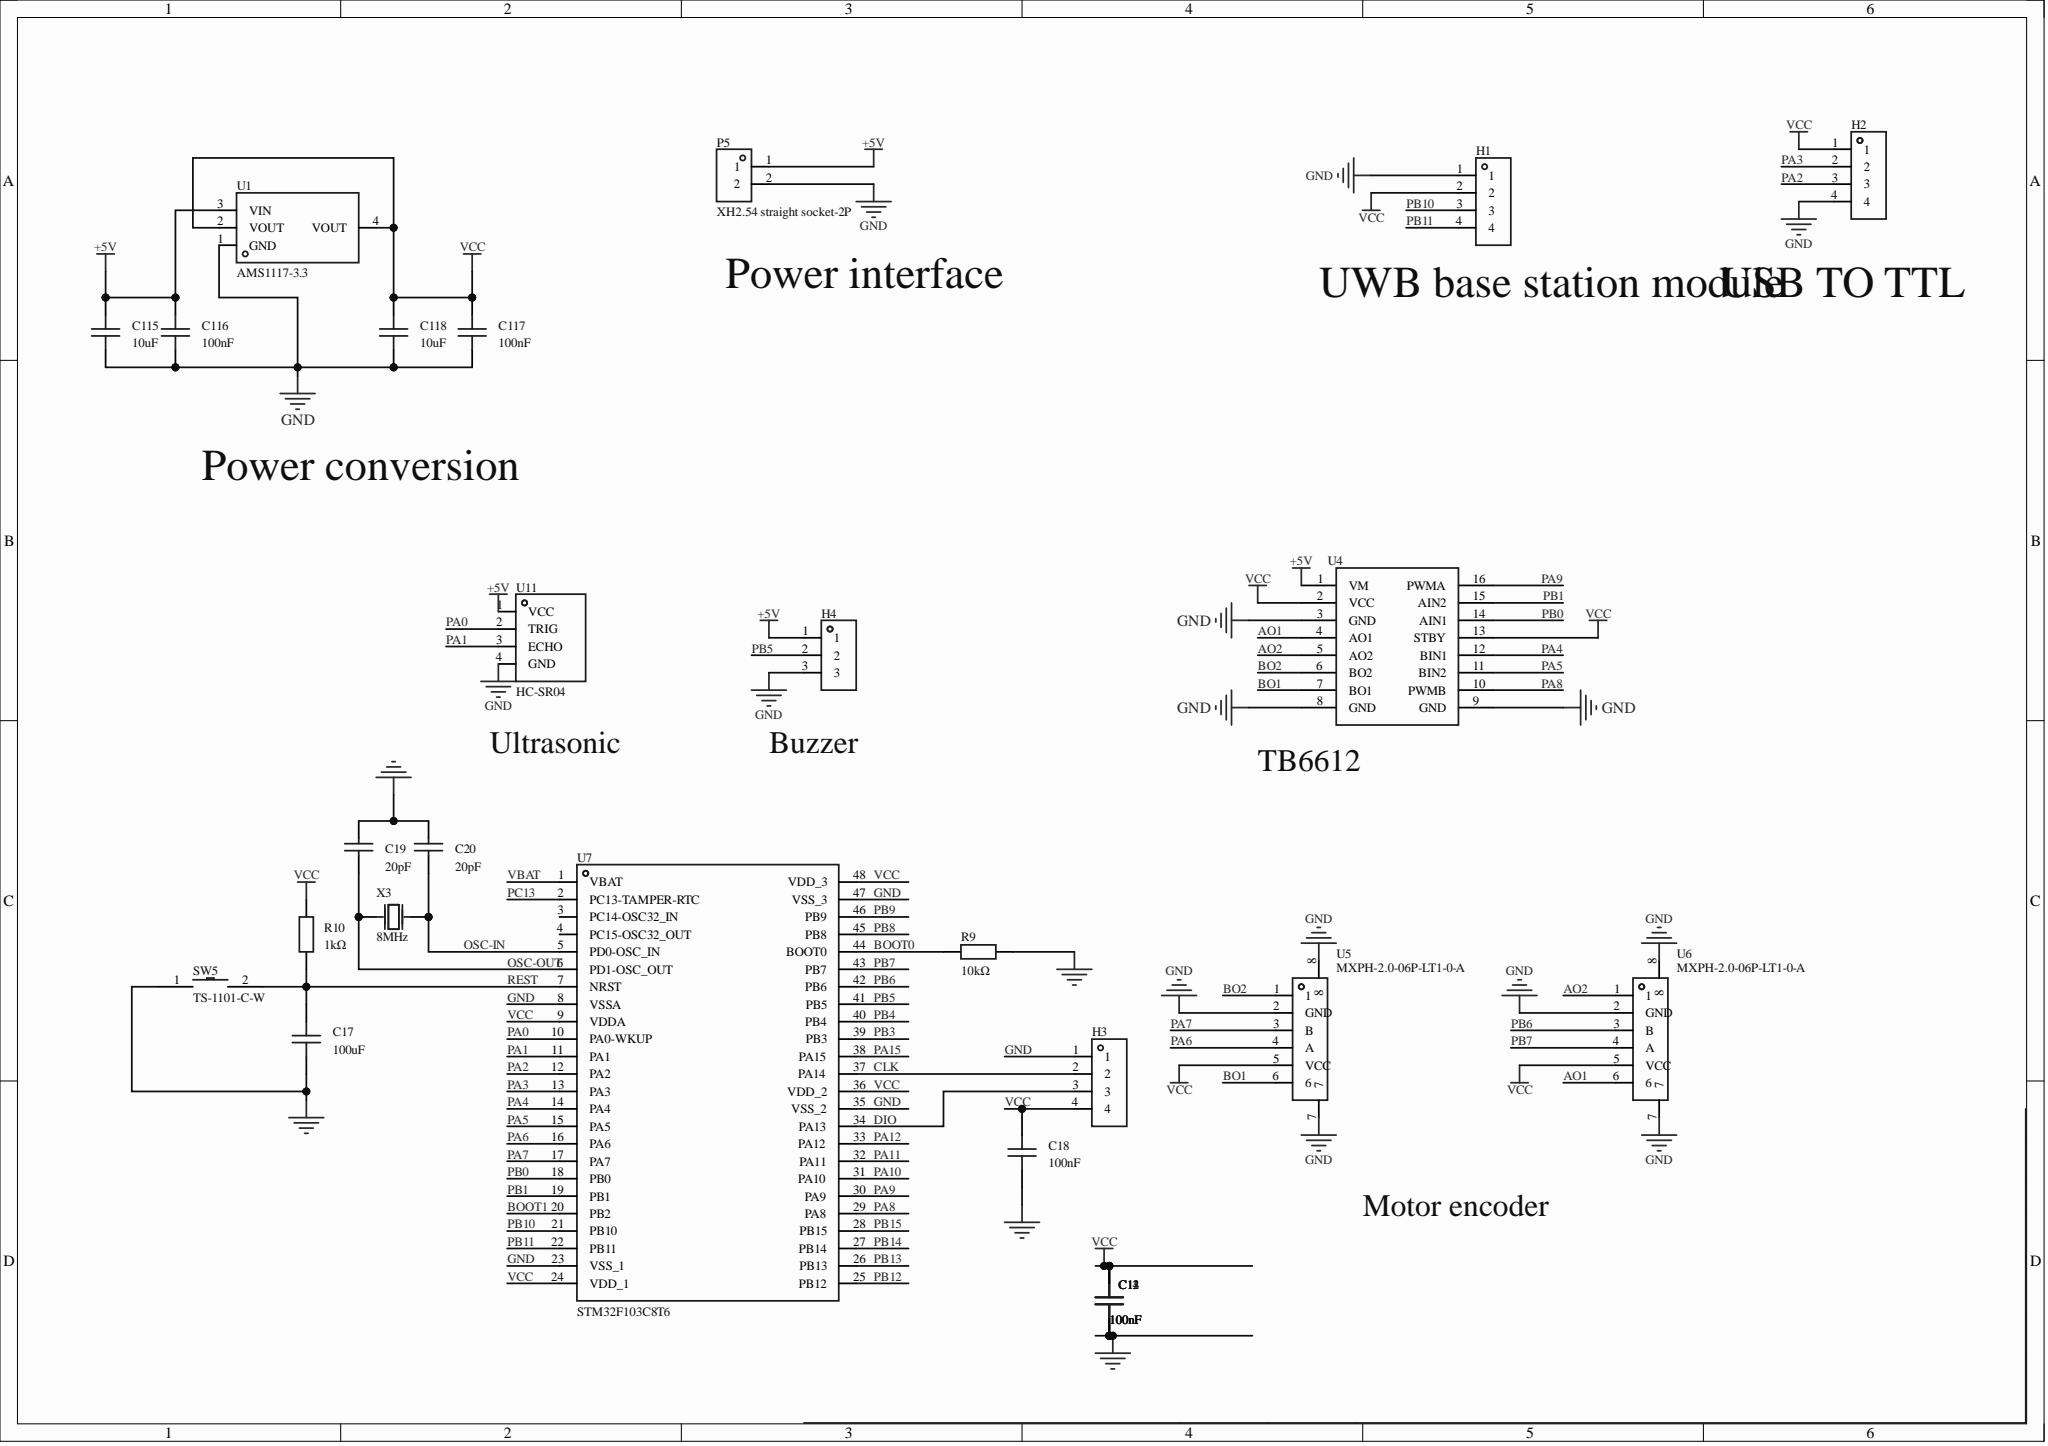Circuit board | Altium Designer | 27 parts | 30 nets
Bill of materials:
Comment,Description,Designator,Footprint,LibRef,Quantity
"100nF","Capacitance: 100nF; tolerance: ±10%; rated voltage: 50V; dielectric (temperature coefficient): X7R;","C11, C12, C13, C14, C18, C116, C117","C0603","CGA0603X7R104K500JT, CC0603KRX7R9BB104","7"
"100uF","Capacitance: 100uF; tolerance: ±20%; rated voltage: 10V; dielectric (temperature coefficient): X5R;","C17","C1206","HGC1206R5107M100NSPJ","1"
"20pF","Capacitance: 20pF; tolerance: ±5%; rated voltage: 50V; dielectric (temperature coefficient): C0G;","C19, C20","C0603","CL10C200JB8NNNC","2"
"10uF","Capacitance: 10uF; tolerance: ±10%; rated voltage: 10V; dielectric (temperature coefficient): X5R;","C115, C118","C0603","CL10A106KP8NNNC","2"
"","","H1, H3","HDR-TH_4P-P2.54-V-M","HDR-M_2.54_1x4P","2"
"","","H2","HDR-TH_4P-P2.54-V-F","HDR-F_2.54_1x4P","1"
"","","H4","HDR-TH_3P-P2.54-V-F","HDR-F_2.54_1x3P","1"
"XH2.54 straight socket-2P","","P5","CONN-TH_XH2.54-2P","XH2.54直插座-2P","1"
"10kΩ","Resistor type: thick film resistor; resistance: 10kΩ; tolerance: ±1%; power: 100mW; max working voltage: 75V; temperature coefficient: ±100ppm/?;","R9","R0603","0603WAF1002T5E","1"
"1kΩ","Resistor type: thick film resistor; resistance: 1kΩ; tolerance: ±1%; power: 100mW; max working voltage: 75V; temperature coefficient: ±100ppm/?;","R10","R0603","RC0603FR-071KL","1"
"TS-1101-C-W","电路结构:单刀单掷;按钮形状:矩形按钮;作用力:260gf;安装方式:立贴;开关长度:6mm;开关宽度:3.6mm;开关高度:2.5mm;带支架:不带;触点电流:50mA;额定电压(AC):-;额定电压(DC):12V;额定功率:-;绝缘电阻:-;带灯:无;机械寿命:5万次;","SW5","SW-SMD_L6.0-W3.3-LS8.0","TS-1101-C-W","1"
"AMS1117-3.3","Output type: fixed; working voltage: -; output voltage: 3.3V; output current: 1A; power supply ripple rejection ratio (PSRR): 72dB@(120Hz); output polarity: positive;","U1","SOT-223-3_L6.5-W3.4-P2.30-LS7.0-BR","AMS1117-3.3_C6186","1"
"","","U4","tb6612","tb6612","1"
"MXPH-2.0-06P-LT1-0-A","插针结构:1x6P;间距:2mm;安装方式:立贴;参考系列:PH;总PIN数:6P;排数:1;每排PIN数:6;额定电流:2A;触头材质:铜合金;触头镀层:锡;工作温度:-25℃~+85℃;","U5, U6","CONN-SMD_6P-P2.00_MXPH-2.0-6P-LT1-0-A","MXPH-2.0-06P-LT1-0-A","2"
"STM32F103C8T6","CPU内核:ARM-M3;程序存储容量:64KB;RAM总容量:20KB;GPIO端口数量:37;工作电压范围:2V~3.6V;CPU最大主频:72MHz;程序存储器类型:FLASH;","U7","LQFP-48_L7.0-W7.0-P0.50-LS9.0-BL","STM32F103C8T6","1"
"HC-SR04","","U11","TH_HC-SR04V","HC-SR04","1"
"8MHz","Crystal type: through-hole crystal; frequency: 8MHz; frequency deviation at room temperature: ±20ppm; external load capacitance: 20pF; frequency stability (full temperature): ±30ppm;","X3","OSC-TH_L10.0-W4.5-P5.00","X49SD8MSD2SC","1"
Netlist (Protel format):
[
C11
C0603
100nF



]
[
C12
C0603
100nF



]
[
C13
C0603
100nF



]
[
C14
C0603
100nF



]
[
C17
C1206
100uF



]
[
C18
C0603
100nF



]
[
C19
C0603
20pF



]
[
C20
C0603
20pF



]
[
C115
C0603
10uF



]
[
C116
C0603
100nF



]
[
C117
C0603
100nF



]
[
C118
C0603
10uF



]
[
H1
HDR-TH_4P-P2.54-V-M




]
[
H2
HDR-TH_4P-P2.54-V-F




]
[
H3
HDR-TH_4P-P2.54-V-M




]
[
H4
HDR-TH_3P-P2.54-V-F




]
[
P5
CONN-TH_XH2.54-2P
XH2.54 straight socket-2P



]
[
R9
R0603
10kΩ



]
[
R10
R0603
1kΩ



]
[
SW5
SW-SMD_L6.0-W3.3-LS8.0
TS-1101-C-W



]
[
U1
SOT-223-3_L6.5-W3.4-P2.30-LS7.0-BR
AMS1117-3.3



]
[
U4
tb6612




]
[
U5
CONN-SMD_6P-P2.00_MXPH-2.0-6P-LT1-0-A
MXPH-2.0-06P-LT1-0-A



]
[
U6
CONN-SMD_6P-P2.00_MXPH-2.0-6P-LT1-0-A
MXPH-2.0-06P-LT1-0-A



]
[
U7
LQFP-48_L7.0-W7.0-P0.50-LS9.0-BL
STM32F103C8T6



]
[
U11
TH_HC-SR04V
HC-SR04



]
[
X3
OSC-TH_L10.0-W4.5-P5.00
8MHz



]
(
VCC
C11-2
C12-2
C13-2
C14-2
C18-2
C117-2
C118-2
H1-2
H2-1
H3-4
R10-2
U1-2
U1-4
U4-2
U4-13
U5-5
U6-5
U7-9
U7-24
U7-36
U7-48
)
(
REST
C17-2
R10-1
SW5-2
U7-7
)
(
PB11
H1-4
U7-22
)
(
PB10
H1-3
U7-21
)
(
PB7
U6-4
U7-43
)
(
PB6
U6-3
U7-42
)
(
PB5
H4-2
U7-41
)
(
PB1
U4-15
U7-19
)
(
PB0
U4-14
U7-18
)
(
PA9
U4-16
U7-30
)
(
PA8
U4-10
U7-29
)
(
PA7
U5-3
U7-17
)
(
PA6
U5-4
U7-16
)
(
PA5
U4-11
U7-15
)
(
PA4
U4-12
U7-14
)
(
PA3
H2-2
U7-13
)
(
PA2
H2-3
U7-12
)
(
PA1
U7-11
U11-3
)
(
PA0
U7-10
U11-2
)
(
OSC-OUT
C19-2
U7-6
X3-2
)
(
OSC-IN
C20-2
U7-5
X3-1
)
(
GND
C11-1
C12-1
C13-1
C14-1
C17-1
C18-1
C19-1
C20-1
C115-1
C116-1
C117-1
C118-1
H1-1
H2-4
H3-1
H4-3
P5-2
R9-1
SW5-1
U1-1
U4-3
U4-8
U4-9
U5-2
U5-7
U5-8
U6-2
U6-7
U6-8
U7-8
U7-23
U7-35
U7-47
U11-4
)
(
DIO
H3-3
U7-34
)
(
CLK
H3-2
U7-37
)
(
BOOT0
R9-2
U7-44
)
(
BO2
U4-6
U5-1
)
(
BO1
U4-7
U5-6
)
(
AO2
U4-5
U6-1
)
(
AO1
U4-4
U6-6
)
(
+5V
C115-2
C116-2
H4-1
P5-1
U1-3
U4-1
U11-1
)